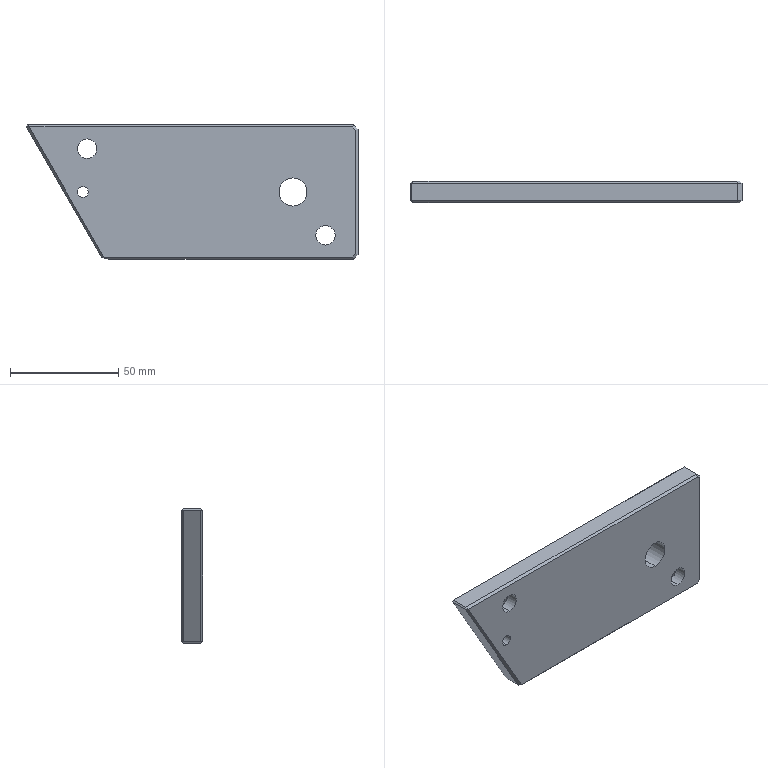Part | STEP file | Placa de deslize - Torre - 1 - 1 cav | 1 solid | 38 faces | box 153.211 x 10 x 62 mm | volume 80124 mm3 | plane 26 | cylinder 8 | cone 4 | commonest cylinder face diameters 9 x4 5 x2 13 x2